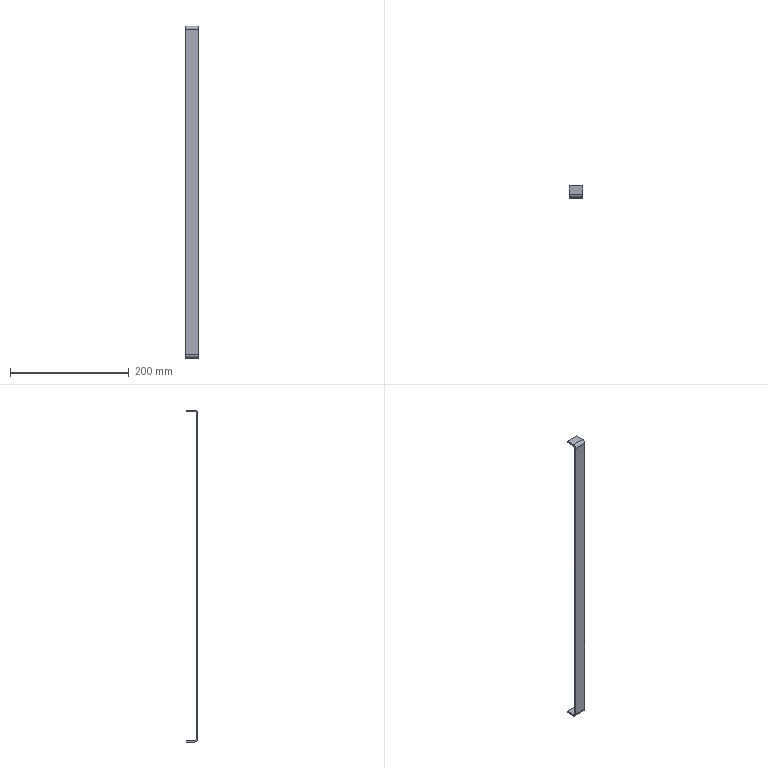Part | SolidWorks | features FlatPattern 1, SMBaseFlange 1, SheetMetal 1 | 1 solid | 22 faces | box 22 x 20 x 560 mm | volume 29947 mm3 | plane 18 | cylinder 4 | commonest cylinder face diameters 6 x2 10.6 x2
STEP:
#1=CARTESIAN_POINT('',(22.,-14.7,0.));
#2=VERTEX_POINT('',#1);
#3=CARTESIAN_POINT('',(22.,-14.7,-2.3));
#4=VERTEX_POINT('',#3);
#5=CARTESIAN_POINT('',(22.,-14.7,0.));
#6=DIRECTION('',(0.,0.,-1.));
#7=VECTOR('',#6,1000.);
#8=LINE('',#5,#7);
#9=EDGE_CURVE('',#2,#4,#8,.T.);
#10=ORIENTED_EDGE('',*,*,#9,.F.);
#11=CARTESIAN_POINT('',(22.,-20.,-5.3));
#12=VERTEX_POINT('',#11);
#13=CARTESIAN_POINT('',(22.,-14.7,-5.3));
#14=DIRECTION('',(1.,0.,0.));
#15=DIRECTION('',(0.,0.,1.));
#16=AXIS2_PLACEMENT_3D('',#13,#14,#15);
#17=CIRCLE('',#16,5.3);
#18=EDGE_CURVE('',#2,#12,#17,.T.);
#19=ORIENTED_EDGE('',*,*,#18,.T.);
#20=CARTESIAN_POINT('',(22.,-17.7,-5.3));
#21=VERTEX_POINT('',#20);
#22=CARTESIAN_POINT('',(22.,-17.7,-5.3));
#23=DIRECTION('',(0.,-1.,0.));
#24=VECTOR('',#23,1000.);
#25=LINE('',#22,#24);
#26=EDGE_CURVE('',#21,#12,#25,.T.);
#27=ORIENTED_EDGE('',*,*,#26,.F.);
#28=CARTESIAN_POINT('',(22.,-14.7,-5.3));
#29=DIRECTION('',(1.,0.,0.));
#30=DIRECTION('',(0.,0.,-1.));
#31=AXIS2_PLACEMENT_3D('',#28,#29,#30);
#32=CIRCLE('',#31,3.);
#33=EDGE_CURVE('',#4,#21,#32,.T.);
#34=ORIENTED_EDGE('',*,*,#33,.F.);
#35=EDGE_LOOP('',(#10,#19,#27,#34));
#36=FACE_OUTER_BOUND('',#35,.T.);
#37=CARTESIAN_POINT('',(22.,-14.7,0.));
#38=DIRECTION('',(1.,0.,0.));
#39=DIRECTION('',(0.,0.,-1.));
#40=AXIS2_PLACEMENT_3D('',#37,#38,#39);
#41=PLANE('',#40);
#42=ADVANCED_FACE('',(#36),#41,.T.);
#43=CARTESIAN_POINT('',(22.,0.,0.));
#44=VERTEX_POINT('',#43);
#45=CARTESIAN_POINT('',(22.,0.,0.));
#46=DIRECTION('',(0.,-1.,0.));
#47=VECTOR('',#46,1000.);
#48=LINE('',#45,#47);
#49=EDGE_CURVE('',#44,#2,#48,.T.);
#50=ORIENTED_EDGE('',*,*,#49,.T.);
#51=ORIENTED_EDGE('',*,*,#9,.T.);
#52=CARTESIAN_POINT('',(22.,0.,-2.3));
#53=VERTEX_POINT('',#52);
#54=CARTESIAN_POINT('',(22.,0.,-2.3));
#55=DIRECTION('',(0.,-1.,0.));
#56=VECTOR('',#55,1000.);
#57=LINE('',#54,#56);
#58=EDGE_CURVE('',#53,#4,#57,.T.);
#59=ORIENTED_EDGE('',*,*,#58,.F.);
#60=CARTESIAN_POINT('',(22.,0.,0.));
#61=DIRECTION('',(0.,0.,-1.));
#62=VECTOR('',#61,1000.);
#63=LINE('',#60,#62);
#64=EDGE_CURVE('',#44,#53,#63,.T.);
#65=ORIENTED_EDGE('',*,*,#64,.F.);
#66=EDGE_LOOP('',(#50,#51,#59,#65));
#67=FACE_OUTER_BOUND('',#66,.T.);
#68=CARTESIAN_POINT('',(22.,-17.7,-5.3));
#69=DIRECTION('',(1.,0.,0.));
#70=DIRECTION('',(0.,0.,-1.));
#71=AXIS2_PLACEMENT_3D('',#68,#69,#70);
#72=PLANE('',#71);
#73=ADVANCED_FACE('',(#67),#72,.T.);
#74=CARTESIAN_POINT('',(0.,-20.,-5.3));
#75=VERTEX_POINT('',#74);
#76=CARTESIAN_POINT('',(0.,-17.7,-5.3));
#77=VERTEX_POINT('',#76);
#78=CARTESIAN_POINT('',(0.,-20.,-5.3));
#79=DIRECTION('',(0.,1.,0.));
#80=VECTOR('',#79,1000.);
#81=LINE('',#78,#80);
#82=EDGE_CURVE('',#75,#77,#81,.T.);
#83=ORIENTED_EDGE('',*,*,#82,.F.);
#84=CARTESIAN_POINT('',(0.,-14.7,0.));
#85=VERTEX_POINT('',#84);
#86=CARTESIAN_POINT('',(0.,-14.7,-5.3));
#87=DIRECTION('',(1.,0.,0.));
#88=DIRECTION('',(0.,0.,1.));
#89=AXIS2_PLACEMENT_3D('',#86,#87,#88);
#90=CIRCLE('',#89,5.3);
#91=EDGE_CURVE('',#85,#75,#90,.T.);
#92=ORIENTED_EDGE('',*,*,#91,.F.);
#93=CARTESIAN_POINT('',(0.,-14.7,-2.3));
#94=VERTEX_POINT('',#93);
#95=CARTESIAN_POINT('',(0.,-14.7,-2.3));
#96=DIRECTION('',(0.,0.,1.));
#97=VECTOR('',#96,1000.);
#98=LINE('',#95,#97);
#99=EDGE_CURVE('',#94,#85,#98,.T.);
#100=ORIENTED_EDGE('',*,*,#99,.F.);
#101=CARTESIAN_POINT('',(0.,-14.7,-5.3));
#102=DIRECTION('',(1.,0.,0.));
#103=DIRECTION('',(0.,0.,-1.));
#104=AXIS2_PLACEMENT_3D('',#101,#102,#103);
#105=CIRCLE('',#104,3.);
#106=EDGE_CURVE('',#94,#77,#105,.T.);
#107=ORIENTED_EDGE('',*,*,#106,.T.);
#108=EDGE_LOOP('',(#83,#92,#100,#107));
#109=FACE_OUTER_BOUND('',#108,.T.);
#110=CARTESIAN_POINT('',(0.,-20.,-5.3));
#111=DIRECTION('',(-1.,0.,0.));
#112=DIRECTION('',(0.,0.,1.));
#113=AXIS2_PLACEMENT_3D('',#110,#111,#112);
#114=PLANE('',#113);
#115=ADVANCED_FACE('',(#109),#114,.T.);
#116=CARTESIAN_POINT('',(0.,-20.,-554.7));
#117=VERTEX_POINT('',#116);
#118=CARTESIAN_POINT('',(0.,-20.,0.));
#119=DIRECTION('',(0.,0.,-1.));
#120=VECTOR('',#119,1000.);
#121=LINE('',#118,#120);
#122=EDGE_CURVE('',#75,#117,#121,.T.);
#123=ORIENTED_EDGE('',*,*,#122,.F.);
#124=ORIENTED_EDGE('',*,*,#82,.T.);
#125=CARTESIAN_POINT('',(0.,-17.7,-554.7));
#126=VERTEX_POINT('',#125);
#127=CARTESIAN_POINT('',(0.,-17.7,0.));
#128=DIRECTION('',(0.,0.,-1.));
#129=VECTOR('',#128,1000.);
#130=LINE('',#127,#129);
#131=EDGE_CURVE('',#77,#126,#130,.T.);
#132=ORIENTED_EDGE('',*,*,#131,.T.);
#133=CARTESIAN_POINT('',(0.,-17.7,-554.7));
#134=DIRECTION('',(0.,-1.,0.));
#135=VECTOR('',#134,1000.);
#136=LINE('',#133,#135);
#137=EDGE_CURVE('',#126,#117,#136,.T.);
#138=ORIENTED_EDGE('',*,*,#137,.T.);
#139=EDGE_LOOP('',(#123,#124,#132,#138));
#140=FACE_OUTER_BOUND('',#139,.T.);
#141=CARTESIAN_POINT('',(0.,-14.7,-2.3));
#142=DIRECTION('',(-1.,0.,0.));
#143=DIRECTION('',(0.,0.,1.));
#144=AXIS2_PLACEMENT_3D('',#141,#142,#143);
#145=PLANE('',#144);
#146=ADVANCED_FACE('',(#140),#145,.T.);
#147=CARTESIAN_POINT('',(22.,-20.,-554.7));
#148=VERTEX_POINT('',#147);
#149=CARTESIAN_POINT('',(22.,-17.7,-554.7));
#150=VERTEX_POINT('',#149);
#151=CARTESIAN_POINT('',(22.,-20.,-554.7));
#152=DIRECTION('',(0.,1.,0.));
#153=VECTOR('',#152,1000.);
#154=LINE('',#151,#153);
#155=EDGE_CURVE('',#148,#150,#154,.T.);
#156=ORIENTED_EDGE('',*,*,#155,.F.);
#157=CARTESIAN_POINT('',(22.,-14.7,-560.));
#158=VERTEX_POINT('',#157);
#159=CARTESIAN_POINT('',(22.,-14.7,-554.7));
#160=DIRECTION('',(1.,0.,0.));
#161=DIRECTION('',(0.,0.,1.));
#162=AXIS2_PLACEMENT_3D('',#159,#160,#161);
#163=CIRCLE('',#162,5.3);
#164=EDGE_CURVE('',#148,#158,#163,.T.);
#165=ORIENTED_EDGE('',*,*,#164,.T.);
#166=CARTESIAN_POINT('',(22.,-14.7,-557.7));
#167=VERTEX_POINT('',#166);
#168=CARTESIAN_POINT('',(22.,-14.7,-557.7));
#169=DIRECTION('',(0.,0.,-1.));
#170=VECTOR('',#169,1000.);
#171=LINE('',#168,#170);
#172=EDGE_CURVE('',#167,#158,#171,.T.);
#173=ORIENTED_EDGE('',*,*,#172,.F.);
#174=CARTESIAN_POINT('',(22.,-14.7,-554.7));
#175=DIRECTION('',(1.,0.,0.));
#176=DIRECTION('',(0.,0.,-1.));
#177=AXIS2_PLACEMENT_3D('',#174,#175,#176);
#178=CIRCLE('',#177,3.);
#179=EDGE_CURVE('',#150,#167,#178,.T.);
#180=ORIENTED_EDGE('',*,*,#179,.F.);
#181=EDGE_LOOP('',(#156,#165,#173,#180));
#182=FACE_OUTER_BOUND('',#181,.T.);
#183=CARTESIAN_POINT('',(22.,-20.,-554.7));
#184=DIRECTION('',(1.,0.,0.));
#185=DIRECTION('',(0.,0.,-1.));
#186=AXIS2_PLACEMENT_3D('',#183,#184,#185);
#187=PLANE('',#186);
#188=ADVANCED_FACE('',(#182),#187,.T.);
#189=CARTESIAN_POINT('',(22.,-20.,0.));
#190=DIRECTION('',(0.,0.,-1.));
#191=VECTOR('',#190,1000.);
#192=LINE('',#189,#191);
#193=EDGE_CURVE('',#12,#148,#192,.T.);
#194=ORIENTED_EDGE('',*,*,#193,.T.);
#195=ORIENTED_EDGE('',*,*,#155,.T.);
#196=CARTESIAN_POINT('',(22.,-17.7,0.));
#197=DIRECTION('',(0.,0.,-1.));
#198=VECTOR('',#197,1000.);
#199=LINE('',#196,#198);
#200=EDGE_CURVE('',#21,#150,#199,.T.);
#201=ORIENTED_EDGE('',*,*,#200,.F.);
#202=ORIENTED_EDGE('',*,*,#26,.T.);
#203=EDGE_LOOP('',(#194,#195,#201,#202));
#204=FACE_OUTER_BOUND('',#203,.T.);
#205=CARTESIAN_POINT('',(22.,-14.7,-557.7));
#206=DIRECTION('',(1.,0.,0.));
#207=DIRECTION('',(0.,0.,-1.));
#208=AXIS2_PLACEMENT_3D('',#205,#206,#207);
#209=PLANE('',#208);
#210=ADVANCED_FACE('',(#204),#209,.T.);
#211=CARTESIAN_POINT('',(0.,-14.7,-560.));
#212=VERTEX_POINT('',#211);
#213=CARTESIAN_POINT('',(0.,-14.7,-557.7));
#214=VERTEX_POINT('',#213);
#215=CARTESIAN_POINT('',(0.,-14.7,-560.));
#216=DIRECTION('',(0.,0.,1.));
#217=VECTOR('',#216,1000.);
#218=LINE('',#215,#217);
#219=EDGE_CURVE('',#212,#214,#218,.T.);
#220=ORIENTED_EDGE('',*,*,#219,.F.);
#221=CARTESIAN_POINT('',(0.,-14.7,-554.7));
#222=DIRECTION('',(1.,0.,0.));
#223=DIRECTION('',(0.,0.,1.));
#224=AXIS2_PLACEMENT_3D('',#221,#222,#223);
#225=CIRCLE('',#224,5.3);
#226=EDGE_CURVE('',#117,#212,#225,.T.);
#227=ORIENTED_EDGE('',*,*,#226,.F.);
#228=ORIENTED_EDGE('',*,*,#137,.F.);
#229=CARTESIAN_POINT('',(0.,-14.7,-554.7));
#230=DIRECTION('',(1.,0.,0.));
#231=DIRECTION('',(0.,0.,-1.));
#232=AXIS2_PLACEMENT_3D('',#229,#230,#231);
#233=CIRCLE('',#232,3.);
#234=EDGE_CURVE('',#126,#214,#233,.T.);
#235=ORIENTED_EDGE('',*,*,#234,.T.);
#236=EDGE_LOOP('',(#220,#227,#228,#235));
#237=FACE_OUTER_BOUND('',#236,.T.);
#238=CARTESIAN_POINT('',(0.,-14.7,-560.));
#239=DIRECTION('',(-1.,0.,0.));
#240=DIRECTION('',(0.,0.,1.));
#241=AXIS2_PLACEMENT_3D('',#238,#239,#240);
#242=PLANE('',#241);
#243=ADVANCED_FACE('',(#237),#242,.T.);
#244=CARTESIAN_POINT('',(0.,0.,-560.));
#245=VERTEX_POINT('',#244);
#246=CARTESIAN_POINT('',(0.,-20.,-560.));
#247=DIRECTION('',(0.,1.,0.));
#248=VECTOR('',#247,1000.);
#249=LINE('',#246,#248);
#250=EDGE_CURVE('',#212,#245,#249,.T.);
#251=ORIENTED_EDGE('',*,*,#250,.F.);
#252=ORIENTED_EDGE('',*,*,#219,.T.);
#253=CARTESIAN_POINT('',(0.,0.,-557.7));
#254=VERTEX_POINT('',#253);
#255=CARTESIAN_POINT('',(0.,-20.,-557.7));
#256=DIRECTION('',(0.,1.,0.));
#257=VECTOR('',#256,1000.);
#258=LINE('',#255,#257);
#259=EDGE_CURVE('',#214,#254,#258,.T.);
#260=ORIENTED_EDGE('',*,*,#259,.T.);
#261=CARTESIAN_POINT('',(0.,0.,-557.7));
#262=DIRECTION('',(0.,0.,-1.));
#263=VECTOR('',#262,1000.);
#264=LINE('',#261,#263);
#265=EDGE_CURVE('',#254,#245,#264,.T.);
#266=ORIENTED_EDGE('',*,*,#265,.T.);
#267=EDGE_LOOP('',(#251,#252,#260,#266));
#268=FACE_OUTER_BOUND('',#267,.T.);
#269=CARTESIAN_POINT('',(0.,-17.7,-554.7));
#270=DIRECTION('',(-1.,0.,0.));
#271=DIRECTION('',(0.,0.,1.));
#272=AXIS2_PLACEMENT_3D('',#269,#270,#271);
#273=PLANE('',#272);
#274=ADVANCED_FACE('',(#268),#273,.T.);
#275=ORIENTED_EDGE('',*,*,#250,.T.);
#276=CARTESIAN_POINT('',(22.,0.,-560.));
#277=VERTEX_POINT('',#276);
#278=CARTESIAN_POINT('',(22.,0.,-560.));
#279=DIRECTION('',(-1.,0.,0.));
#280=VECTOR('',#279,1000.);
#281=LINE('',#278,#280);
#282=EDGE_CURVE('',#277,#245,#281,.T.);
#283=ORIENTED_EDGE('',*,*,#282,.F.);
#284=CARTESIAN_POINT('',(22.,-20.,-560.));
#285=DIRECTION('',(0.,1.,0.));
#286=VECTOR('',#285,1000.);
#287=LINE('',#284,#286);
#288=EDGE_CURVE('',#158,#277,#287,.T.);
#289=ORIENTED_EDGE('',*,*,#288,.F.);
#290=CARTESIAN_POINT('',(22.,-14.7,-560.));
#291=DIRECTION('',(-1.,0.,0.));
#292=VECTOR('',#291,1000.);
#293=LINE('',#290,#292);
#294=EDGE_CURVE('',#158,#212,#293,.T.);
#295=ORIENTED_EDGE('',*,*,#294,.T.);
#296=EDGE_LOOP('',(#275,#283,#289,#295));
#297=FACE_OUTER_BOUND('',#296,.T.);
#298=CARTESIAN_POINT('',(22.,-20.,-560.));
#299=DIRECTION('',(0.,0.,1.));
#300=DIRECTION('',(1.,0.,0.));
#301=AXIS2_PLACEMENT_3D('',#298,#299,#300);
#302=PLANE('',#301);
#303=ADVANCED_FACE('',(#297),#302,.F.);
#304=ORIENTED_EDGE('',*,*,#265,.F.);
#305=CARTESIAN_POINT('',(22.,0.,-557.7));
#306=VERTEX_POINT('',#305);
#307=CARTESIAN_POINT('',(22.,0.,-557.7));
#308=DIRECTION('',(-1.,0.,0.));
#309=VECTOR('',#308,1000.);
#310=LINE('',#307,#309);
#311=EDGE_CURVE('',#306,#254,#310,.T.);
#312=ORIENTED_EDGE('',*,*,#311,.F.);
#313=CARTESIAN_POINT('',(22.,0.,-557.7));
#314=DIRECTION('',(0.,0.,-1.));
#315=VECTOR('',#314,1000.);
#316=LINE('',#313,#315);
#317=EDGE_CURVE('',#306,#277,#316,.T.);
#318=ORIENTED_EDGE('',*,*,#317,.T.);
#319=ORIENTED_EDGE('',*,*,#282,.T.);
#320=EDGE_LOOP('',(#304,#312,#318,#319));
#321=FACE_OUTER_BOUND('',#320,.T.);
#322=CARTESIAN_POINT('',(22.,0.,-557.7));
#323=DIRECTION('',(0.,1.,0.));
#324=DIRECTION('',(0.,0.,1.));
#325=AXIS2_PLACEMENT_3D('',#322,#323,#324);
#326=PLANE('',#325);
#327=ADVANCED_FACE('',(#321),#326,.T.);
#328=ORIENTED_EDGE('',*,*,#259,.F.);
#329=CARTESIAN_POINT('',(22.,-14.7,-557.7));
#330=DIRECTION('',(-1.,0.,0.));
#331=VECTOR('',#330,1000.);
#332=LINE('',#329,#331);
#333=EDGE_CURVE('',#167,#214,#332,.T.);
#334=ORIENTED_EDGE('',*,*,#333,.F.);
#335=CARTESIAN_POINT('',(22.,-20.,-557.7));
#336=DIRECTION('',(0.,1.,0.));
#337=VECTOR('',#336,1000.);
#338=LINE('',#335,#337);
#339=EDGE_CURVE('',#167,#306,#338,.T.);
#340=ORIENTED_EDGE('',*,*,#339,.T.);
#341=ORIENTED_EDGE('',*,*,#311,.T.);
#342=EDGE_LOOP('',(#328,#334,#340,#341));
#343=FACE_OUTER_BOUND('',#342,.T.);
#344=CARTESIAN_POINT('',(22.,-20.,-557.7));
#345=DIRECTION('',(0.,0.,1.));
#346=DIRECTION('',(1.,0.,0.));
#347=AXIS2_PLACEMENT_3D('',#344,#345,#346);
#348=PLANE('',#347);
#349=ADVANCED_FACE('',(#343),#348,.T.);
#350=ORIENTED_EDGE('',*,*,#234,.F.);
#351=CARTESIAN_POINT('',(22.,-17.7,-554.7));
#352=DIRECTION('',(-1.,0.,0.));
#353=VECTOR('',#352,1000.);
#354=LINE('',#351,#353);
#355=EDGE_CURVE('',#150,#126,#354,.T.);
#356=ORIENTED_EDGE('',*,*,#355,.F.);
#357=ORIENTED_EDGE('',*,*,#179,.T.);
#358=ORIENTED_EDGE('',*,*,#333,.T.);
#359=EDGE_LOOP('',(#350,#356,#357,#358));
#360=FACE_OUTER_BOUND('',#359,.T.);
#361=CARTESIAN_POINT('',(22.,-14.7,-554.7));
#362=DIRECTION('',(-1.,0.,0.));
#363=DIRECTION('',(0.,0.,1.));
#364=AXIS2_PLACEMENT_3D('',#361,#362,#363);
#365=CYLINDRICAL_SURFACE('',#364,3.);
#366=ADVANCED_FACE('',(#360),#365,.F.);
#367=ORIENTED_EDGE('',*,*,#131,.F.);
#368=CARTESIAN_POINT('',(22.,-17.7,-5.3));
#369=DIRECTION('',(-1.,0.,0.));
#370=VECTOR('',#369,1000.);
#371=LINE('',#368,#370);
#372=EDGE_CURVE('',#21,#77,#371,.T.);
#373=ORIENTED_EDGE('',*,*,#372,.F.);
#374=ORIENTED_EDGE('',*,*,#200,.T.);
#375=ORIENTED_EDGE('',*,*,#355,.T.);
#376=EDGE_LOOP('',(#367,#373,#374,#375));
#377=FACE_OUTER_BOUND('',#376,.T.);
#378=CARTESIAN_POINT('',(22.,-17.7,0.));
#379=DIRECTION('',(0.,1.,0.));
#380=DIRECTION('',(0.,0.,1.));
#381=AXIS2_PLACEMENT_3D('',#378,#379,#380);
#382=PLANE('',#381);
#383=ADVANCED_FACE('',(#377),#382,.T.);
#384=ORIENTED_EDGE('',*,*,#106,.F.);
#385=CARTESIAN_POINT('',(22.,-14.7,-2.3));
#386=DIRECTION('',(-1.,0.,0.));
#387=VECTOR('',#386,1000.);
#388=LINE('',#385,#387);
#389=EDGE_CURVE('',#4,#94,#388,.T.);
#390=ORIENTED_EDGE('',*,*,#389,.F.);
#391=ORIENTED_EDGE('',*,*,#33,.T.);
#392=ORIENTED_EDGE('',*,*,#372,.T.);
#393=EDGE_LOOP('',(#384,#390,#391,#392));
#394=FACE_OUTER_BOUND('',#393,.T.);
#395=CARTESIAN_POINT('',(22.,-14.7,-5.3));
#396=DIRECTION('',(-1.,0.,0.));
#397=DIRECTION('',(0.,0.,1.));
#398=AXIS2_PLACEMENT_3D('',#395,#396,#397);
#399=CYLINDRICAL_SURFACE('',#398,3.);
#400=ADVANCED_FACE('',(#394),#399,.F.);
#401=CARTESIAN_POINT('',(0.,0.,-2.3));
#402=VERTEX_POINT('',#401);
#403=CARTESIAN_POINT('',(0.,0.,-2.3));
#404=DIRECTION('',(0.,-1.,0.));
#405=VECTOR('',#404,1000.);
#406=LINE('',#403,#405);
#407=EDGE_CURVE('',#402,#94,#406,.T.);
#408=ORIENTED_EDGE('',*,*,#407,.F.);
#409=CARTESIAN_POINT('',(22.,0.,-2.3));
#410=DIRECTION('',(-1.,0.,0.));
#411=VECTOR('',#410,1000.);
#412=LINE('',#409,#411);
#413=EDGE_CURVE('',#53,#402,#412,.T.);
#414=ORIENTED_EDGE('',*,*,#413,.F.);
#415=ORIENTED_EDGE('',*,*,#58,.T.);
#416=ORIENTED_EDGE('',*,*,#389,.T.);
#417=EDGE_LOOP('',(#408,#414,#415,#416));
#418=FACE_OUTER_BOUND('',#417,.T.);
#419=CARTESIAN_POINT('',(22.,0.,-2.3));
#420=DIRECTION('',(0.,0.,-1.));
#421=DIRECTION('',(-1.,0.,0.));
#422=AXIS2_PLACEMENT_3D('',#419,#420,#421);
#423=PLANE('',#422);
#424=ADVANCED_FACE('',(#418),#423,.T.);
#425=CARTESIAN_POINT('',(0.,0.,0.));
#426=VERTEX_POINT('',#425);
#427=CARTESIAN_POINT('',(0.,0.,0.));
#428=DIRECTION('',(0.,0.,-1.));
#429=VECTOR('',#428,1000.);
#430=LINE('',#427,#429);
#431=EDGE_CURVE('',#426,#402,#430,.T.);
#432=ORIENTED_EDGE('',*,*,#431,.F.);
#433=CARTESIAN_POINT('',(22.,0.,0.));
#434=DIRECTION('',(-1.,0.,0.));
#435=VECTOR('',#434,1000.);
#436=LINE('',#433,#435);
#437=EDGE_CURVE('',#44,#426,#436,.T.);
#438=ORIENTED_EDGE('',*,*,#437,.F.);
#439=ORIENTED_EDGE('',*,*,#64,.T.);
#440=ORIENTED_EDGE('',*,*,#413,.T.);
#441=EDGE_LOOP('',(#432,#438,#439,#440));
#442=FACE_OUTER_BOUND('',#441,.T.);
#443=CARTESIAN_POINT('',(22.,0.,0.));
#444=DIRECTION('',(0.,1.,0.));
#445=DIRECTION('',(0.,0.,1.));
#446=AXIS2_PLACEMENT_3D('',#443,#444,#445);
#447=PLANE('',#446);
#448=ADVANCED_FACE('',(#442),#447,.T.);
#449=CARTESIAN_POINT('',(0.,0.,0.));
#450=DIRECTION('',(0.,-1.,0.));
#451=VECTOR('',#450,1000.);
#452=LINE('',#449,#451);
#453=EDGE_CURVE('',#426,#85,#452,.T.);
#454=ORIENTED_EDGE('',*,*,#453,.T.);
#455=CARTESIAN_POINT('',(22.,-14.7,0.));
#456=DIRECTION('',(-1.,0.,0.));
#457=VECTOR('',#456,1000.);
#458=LINE('',#455,#457);
#459=EDGE_CURVE('',#2,#85,#458,.T.);
#460=ORIENTED_EDGE('',*,*,#459,.F.);
#461=ORIENTED_EDGE('',*,*,#49,.F.);
#462=ORIENTED_EDGE('',*,*,#437,.T.);
#463=EDGE_LOOP('',(#454,#460,#461,#462));
#464=FACE_OUTER_BOUND('',#463,.T.);
#465=CARTESIAN_POINT('',(22.,0.,0.));
#466=DIRECTION('',(0.,0.,-1.));
#467=DIRECTION('',(-1.,0.,0.));
#468=AXIS2_PLACEMENT_3D('',#465,#466,#467);
#469=PLANE('',#468);
#470=ADVANCED_FACE('',(#464),#469,.F.);
#471=ORIENTED_EDGE('',*,*,#91,.T.);
#472=CARTESIAN_POINT('',(22.,-20.,-5.3));
#473=DIRECTION('',(-1.,0.,0.));
#474=VECTOR('',#473,1000.);
#475=LINE('',#472,#474);
#476=EDGE_CURVE('',#12,#75,#475,.T.);
#477=ORIENTED_EDGE('',*,*,#476,.F.);
#478=ORIENTED_EDGE('',*,*,#18,.F.);
#479=ORIENTED_EDGE('',*,*,#459,.T.);
#480=EDGE_LOOP('',(#471,#477,#478,#479));
#481=FACE_OUTER_BOUND('',#480,.T.);
#482=CARTESIAN_POINT('',(22.,-14.7,-5.3));
#483=DIRECTION('',(-1.,0.,0.));
#484=DIRECTION('',(0.,0.,1.));
#485=AXIS2_PLACEMENT_3D('',#482,#483,#484);
#486=CYLINDRICAL_SURFACE('',#485,5.3);
#487=ADVANCED_FACE('',(#481),#486,.T.);
#488=ORIENTED_EDGE('',*,*,#122,.T.);
#489=CARTESIAN_POINT('',(22.,-20.,-554.7));
#490=DIRECTION('',(-1.,0.,0.));
#491=VECTOR('',#490,1000.);
#492=LINE('',#489,#491);
#493=EDGE_CURVE('',#148,#117,#492,.T.);
#494=ORIENTED_EDGE('',*,*,#493,.F.);
#495=ORIENTED_EDGE('',*,*,#193,.F.);
#496=ORIENTED_EDGE('',*,*,#476,.T.);
#497=EDGE_LOOP('',(#488,#494,#495,#496));
#498=FACE_OUTER_BOUND('',#497,.T.);
#499=CARTESIAN_POINT('',(22.,-20.,0.));
#500=DIRECTION('',(0.,1.,0.));
#501=DIRECTION('',(0.,0.,1.));
#502=AXIS2_PLACEMENT_3D('',#499,#500,#501);
#503=PLANE('',#502);
#504=ADVANCED_FACE('',(#498),#503,.F.);
#505=ORIENTED_EDGE('',*,*,#226,.T.);
#506=ORIENTED_EDGE('',*,*,#294,.F.);
#507=ORIENTED_EDGE('',*,*,#164,.F.);
#508=ORIENTED_EDGE('',*,*,#493,.T.);
#509=EDGE_LOOP('',(#505,#506,#507,#508));
#510=FACE_OUTER_BOUND('',#509,.T.);
#511=CARTESIAN_POINT('',(22.,-14.7,-554.7));
#512=DIRECTION('',(-1.,0.,0.));
#513=DIRECTION('',(0.,0.,1.));
#514=AXIS2_PLACEMENT_3D('',#511,#512,#513);
#515=CYLINDRICAL_SURFACE('',#514,5.3);
#516=ADVANCED_FACE('',(#510),#515,.T.);
#517=ORIENTED_EDGE('',*,*,#288,.T.);
#518=ORIENTED_EDGE('',*,*,#317,.F.);
#519=ORIENTED_EDGE('',*,*,#339,.F.);
#520=ORIENTED_EDGE('',*,*,#172,.T.);
#521=EDGE_LOOP('',(#517,#518,#519,#520));
#522=FACE_OUTER_BOUND('',#521,.T.);
#523=CARTESIAN_POINT('',(22.,-14.7,-554.7));
#524=DIRECTION('',(1.,0.,0.));
#525=DIRECTION('',(0.,0.,-1.));
#526=AXIS2_PLACEMENT_3D('',#523,#524,#525);
#527=PLANE('',#526);
#528=ADVANCED_FACE('',(#522),#527,.T.);
#529=ORIENTED_EDGE('',*,*,#407,.T.);
#530=ORIENTED_EDGE('',*,*,#99,.T.);
#531=ORIENTED_EDGE('',*,*,#453,.F.);
#532=ORIENTED_EDGE('',*,*,#431,.T.);
#533=EDGE_LOOP('',(#529,#530,#531,#532));
#534=FACE_OUTER_BOUND('',#533,.T.);
#535=CARTESIAN_POINT('',(0.,-14.7,-554.7));
#536=DIRECTION('',(1.,0.,0.));
#537=DIRECTION('',(0.,0.,-1.));
#538=AXIS2_PLACEMENT_3D('',#535,#536,#537);
#539=PLANE('',#538);
#540=ADVANCED_FACE('',(#534),#539,.F.);
#541=CLOSED_SHELL('',(#42,#73,#115,#146,#188,#210,#243,#274,#303,#327,#349,#366,#383,#400,#424,#448,#470,#487,#504,#516,#528,#540));
#542=MANIFOLD_SOLID_BREP('',#541);
#543=CARTESIAN_POINT('',(0.,0.,0.));
#544=DIRECTION('',(0.,0.,1.));
#545=DIRECTION('',(1.,0.,0.));
#546=AXIS2_PLACEMENT_3D('',#543,#544,#545);
#547=(LENGTH_UNIT()NAMED_UNIT(*)SI_UNIT(.MILLI.,.METRE.));
#548=UNCERTAINTY_MEASURE_WITH_UNIT(LENGTH_MEASURE(0.00001),#547,'','');
#549=(NAMED_UNIT(*)PLANE_ANGLE_UNIT()SI_UNIT($,.RADIAN.));
#550=(NAMED_UNIT(*)SI_UNIT($,.STERADIAN.)SOLID_ANGLE_UNIT());
#551=(GEOMETRIC_REPRESENTATION_CONTEXT(3)GLOBAL_UNCERTAINTY_ASSIGNED_CONTEXT((#548))GLOBAL_UNIT_ASSIGNED_CONTEXT((#547,#549,#550))REPRESENTATION_CONTEXT('',''));
#552=ADVANCED_BREP_SHAPE_REPRESENTATION('',(#542,#546),#551);